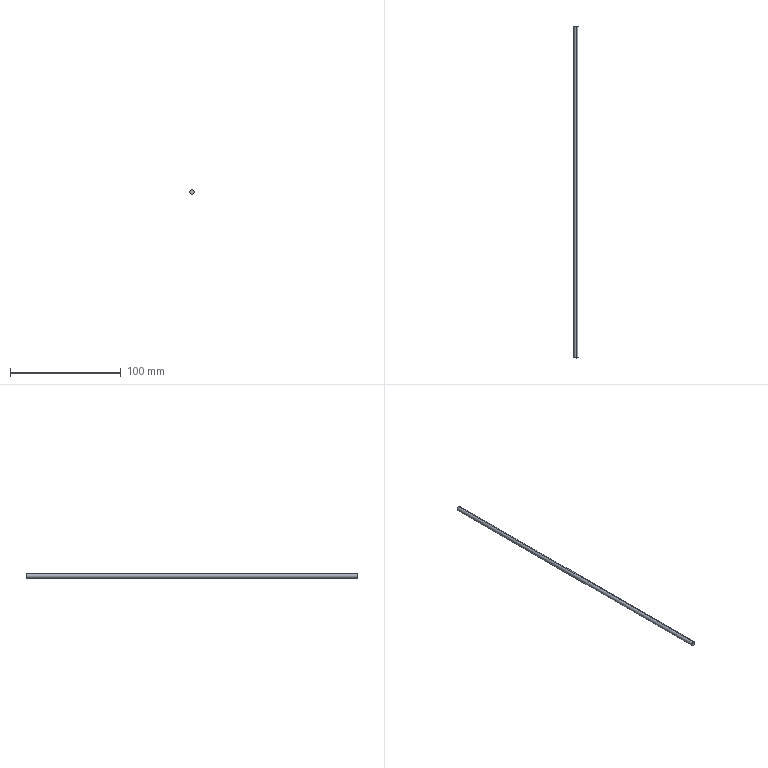Part | SolidWorks | features Extrusion 1 | 1 solid | 4 faces | box 4 x 300 x 4 mm | volume 3770 mm3 | cylinder 2 | plane 2 | commonest cylinder face diameters 4 x2
STEP:
#1=CARTESIAN_POINT('',(0.,300.,2.));
#2=VERTEX_POINT('',#1);
#3=CARTESIAN_POINT('',(0.,300.,-2.));
#4=VERTEX_POINT('',#3);
#5=CARTESIAN_POINT('',(0.,300.,0.));
#6=DIRECTION('',(0.,1.,0.));
#7=DIRECTION('',(0.,0.,1.));
#8=AXIS2_PLACEMENT_3D('',#5,#6,#7);
#9=CIRCLE('',#8,2.);
#10=EDGE_CURVE('',#2,#4,#9,.T.);
#11=ORIENTED_EDGE('',*,*,#10,.F.);
#12=CARTESIAN_POINT('',(0.,0.,2.));
#13=VERTEX_POINT('',#12);
#14=CARTESIAN_POINT('',(0.,300.,2.));
#15=DIRECTION('',(0.,-1.,0.));
#16=VECTOR('',#15,1000.);
#17=LINE('',#14,#16);
#18=EDGE_CURVE('',#2,#13,#17,.T.);
#19=ORIENTED_EDGE('',*,*,#18,.T.);
#20=CARTESIAN_POINT('',(0.,0.,-2.));
#21=VERTEX_POINT('',#20);
#22=CARTESIAN_POINT('',(0.,0.,0.));
#23=DIRECTION('',(0.,1.,0.));
#24=DIRECTION('',(0.,0.,1.));
#25=AXIS2_PLACEMENT_3D('',#22,#23,#24);
#26=CIRCLE('',#25,2.);
#27=EDGE_CURVE('',#13,#21,#26,.T.);
#28=ORIENTED_EDGE('',*,*,#27,.T.);
#29=CARTESIAN_POINT('',(0.,300.,-2.));
#30=DIRECTION('',(0.,-1.,0.));
#31=VECTOR('',#30,1000.);
#32=LINE('',#29,#31);
#33=EDGE_CURVE('',#4,#21,#32,.T.);
#34=ORIENTED_EDGE('',*,*,#33,.F.);
#35=EDGE_LOOP('',(#11,#19,#28,#34));
#36=FACE_OUTER_BOUND('',#35,.T.);
#37=CARTESIAN_POINT('',(0.,300.,0.));
#38=DIRECTION('',(0.,-1.,0.));
#39=DIRECTION('',(0.,0.,-1.));
#40=AXIS2_PLACEMENT_3D('',#37,#38,#39);
#41=CYLINDRICAL_SURFACE('',#40,2.);
#42=ADVANCED_FACE('',(#36),#41,.T.);
#43=ORIENTED_EDGE('',*,*,#18,.F.);
#44=CARTESIAN_POINT('',(0.,300.,0.));
#45=DIRECTION('',(0.,1.,0.));
#46=DIRECTION('',(0.,0.,1.));
#47=AXIS2_PLACEMENT_3D('',#44,#45,#46);
#48=CIRCLE('',#47,2.);
#49=EDGE_CURVE('',#4,#2,#48,.T.);
#50=ORIENTED_EDGE('',*,*,#49,.F.);
#51=ORIENTED_EDGE('',*,*,#33,.T.);
#52=CARTESIAN_POINT('',(0.,0.,0.));
#53=DIRECTION('',(0.,1.,0.));
#54=DIRECTION('',(0.,0.,1.));
#55=AXIS2_PLACEMENT_3D('',#52,#53,#54);
#56=CIRCLE('',#55,2.);
#57=EDGE_CURVE('',#21,#13,#56,.T.);
#58=ORIENTED_EDGE('',*,*,#57,.T.);
#59=EDGE_LOOP('',(#43,#50,#51,#58));
#60=FACE_OUTER_BOUND('',#59,.T.);
#61=CARTESIAN_POINT('',(0.,300.,0.));
#62=DIRECTION('',(0.,-1.,0.));
#63=DIRECTION('',(0.,0.,-1.));
#64=AXIS2_PLACEMENT_3D('',#61,#62,#63);
#65=CYLINDRICAL_SURFACE('',#64,2.);
#66=ADVANCED_FACE('',(#60),#65,.T.);
#67=ORIENTED_EDGE('',*,*,#49,.T.);
#68=ORIENTED_EDGE('',*,*,#10,.T.);
#69=EDGE_LOOP('',(#67,#68));
#70=FACE_OUTER_BOUND('',#69,.T.);
#71=CARTESIAN_POINT('',(0.,300.,0.));
#72=DIRECTION('',(0.,1.,0.));
#73=DIRECTION('',(0.,0.,1.));
#74=AXIS2_PLACEMENT_3D('',#71,#72,#73);
#75=PLANE('',#74);
#76=ADVANCED_FACE('',(#70),#75,.T.);
#77=ORIENTED_EDGE('',*,*,#57,.F.);
#78=ORIENTED_EDGE('',*,*,#27,.F.);
#79=EDGE_LOOP('',(#77,#78));
#80=FACE_OUTER_BOUND('',#79,.T.);
#81=CARTESIAN_POINT('',(0.,0.,0.));
#82=DIRECTION('',(0.,1.,0.));
#83=DIRECTION('',(0.,0.,1.));
#84=AXIS2_PLACEMENT_3D('',#81,#82,#83);
#85=PLANE('',#84);
#86=ADVANCED_FACE('',(#80),#85,.F.);
#87=CLOSED_SHELL('',(#42,#66,#76,#86));
#88=MANIFOLD_SOLID_BREP('',#87);
#89=CARTESIAN_POINT('',(0.,0.,0.));
#90=DIRECTION('',(0.,0.,1.));
#91=DIRECTION('',(1.,0.,0.));
#92=AXIS2_PLACEMENT_3D('',#89,#90,#91);
#93=(LENGTH_UNIT()NAMED_UNIT(*)SI_UNIT(.MILLI.,.METRE.));
#94=UNCERTAINTY_MEASURE_WITH_UNIT(LENGTH_MEASURE(0.00001),#93,'','');
#95=(NAMED_UNIT(*)PLANE_ANGLE_UNIT()SI_UNIT($,.RADIAN.));
#96=(NAMED_UNIT(*)SI_UNIT($,.STERADIAN.)SOLID_ANGLE_UNIT());
#97=(GEOMETRIC_REPRESENTATION_CONTEXT(3)GLOBAL_UNCERTAINTY_ASSIGNED_CONTEXT((#94))GLOBAL_UNIT_ASSIGNED_CONTEXT((#93,#95,#96))REPRESENTATION_CONTEXT('',''));
#98=ADVANCED_BREP_SHAPE_REPRESENTATION('',(#88,#92),#97);